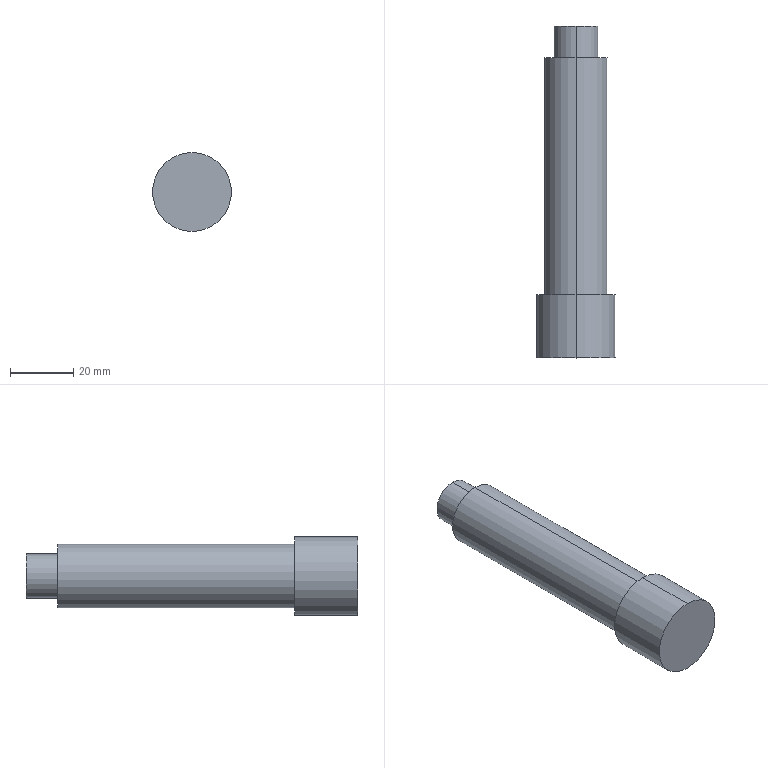Part | SolidWorks | features ICE 2, Extrusion 1 | 1 solid | 10 faces | box 25 x 105 x 25 mm | volume 34919 mm3 | cylinder 6 | plane 4 | commonest cylinder face diameters 14 x2 20 x2 25 x2
STEP:
#1=CARTESIAN_POINT('',(0.,105.,7.));
#2=VERTEX_POINT('',#1);
#3=CARTESIAN_POINT('',(0.,105.,-7.));
#4=VERTEX_POINT('',#3);
#5=CARTESIAN_POINT('',(0.,105.,0.));
#6=DIRECTION('',(0.,1.,0.));
#7=DIRECTION('',(0.,0.,1.));
#8=AXIS2_PLACEMENT_3D('',#5,#6,#7);
#9=CIRCLE('',#8,7.);
#10=EDGE_CURVE('',#2,#4,#9,.T.);
#11=ORIENTED_EDGE('',*,*,#10,.F.);
#12=CARTESIAN_POINT('',(0.,95.,7.));
#13=VERTEX_POINT('',#12);
#14=CARTESIAN_POINT('',(0.,105.,7.));
#15=DIRECTION('',(0.,-1.,0.));
#16=VECTOR('',#15,1000.);
#17=LINE('',#14,#16);
#18=EDGE_CURVE('',#2,#13,#17,.T.);
#19=ORIENTED_EDGE('',*,*,#18,.T.);
#20=CARTESIAN_POINT('',(0.,95.,-7.));
#21=VERTEX_POINT('',#20);
#22=CARTESIAN_POINT('',(0.,95.,0.));
#23=DIRECTION('',(0.,1.,0.));
#24=DIRECTION('',(0.,0.,1.));
#25=AXIS2_PLACEMENT_3D('',#22,#23,#24);
#26=CIRCLE('',#25,7.);
#27=EDGE_CURVE('',#13,#21,#26,.T.);
#28=ORIENTED_EDGE('',*,*,#27,.T.);
#29=CARTESIAN_POINT('',(0.,105.,-7.));
#30=DIRECTION('',(0.,-1.,0.));
#31=VECTOR('',#30,1000.);
#32=LINE('',#29,#31);
#33=EDGE_CURVE('',#4,#21,#32,.T.);
#34=ORIENTED_EDGE('',*,*,#33,.F.);
#35=EDGE_LOOP('',(#11,#19,#28,#34));
#36=FACE_OUTER_BOUND('',#35,.T.);
#37=CARTESIAN_POINT('',(0.,105.,0.));
#38=DIRECTION('',(0.,-1.,0.));
#39=DIRECTION('',(0.,0.,-1.));
#40=AXIS2_PLACEMENT_3D('',#37,#38,#39);
#41=CYLINDRICAL_SURFACE('',#40,7.);
#42=ADVANCED_FACE('',(#36),#41,.T.);
#43=CARTESIAN_POINT('',(0.,95.,10.));
#44=VERTEX_POINT('',#43);
#45=CARTESIAN_POINT('',(0.,95.,-10.));
#46=VERTEX_POINT('',#45);
#47=CARTESIAN_POINT('',(0.,95.,0.));
#48=DIRECTION('',(0.,1.,0.));
#49=DIRECTION('',(0.,0.,1.));
#50=AXIS2_PLACEMENT_3D('',#47,#48,#49);
#51=CIRCLE('',#50,10.);
#52=EDGE_CURVE('',#44,#46,#51,.T.);
#53=ORIENTED_EDGE('',*,*,#52,.F.);
#54=CARTESIAN_POINT('',(0.,20.,10.));
#55=VERTEX_POINT('',#54);
#56=CARTESIAN_POINT('',(0.,95.,10.));
#57=DIRECTION('',(0.,-1.,0.));
#58=VECTOR('',#57,1000.);
#59=LINE('',#56,#58);
#60=EDGE_CURVE('',#44,#55,#59,.T.);
#61=ORIENTED_EDGE('',*,*,#60,.T.);
#62=CARTESIAN_POINT('',(0.,20.,-10.));
#63=VERTEX_POINT('',#62);
#64=CARTESIAN_POINT('',(0.,20.,0.));
#65=DIRECTION('',(0.,1.,0.));
#66=DIRECTION('',(0.,0.,1.));
#67=AXIS2_PLACEMENT_3D('',#64,#65,#66);
#68=CIRCLE('',#67,10.);
#69=EDGE_CURVE('',#55,#63,#68,.T.);
#70=ORIENTED_EDGE('',*,*,#69,.T.);
#71=CARTESIAN_POINT('',(0.,95.,-10.));
#72=DIRECTION('',(0.,-1.,0.));
#73=VECTOR('',#72,1000.);
#74=LINE('',#71,#73);
#75=EDGE_CURVE('',#46,#63,#74,.T.);
#76=ORIENTED_EDGE('',*,*,#75,.F.);
#77=EDGE_LOOP('',(#53,#61,#70,#76));
#78=FACE_OUTER_BOUND('',#77,.T.);
#79=CARTESIAN_POINT('',(0.,95.,0.));
#80=DIRECTION('',(0.,-1.,0.));
#81=DIRECTION('',(0.,0.,-1.));
#82=AXIS2_PLACEMENT_3D('',#79,#80,#81);
#83=CYLINDRICAL_SURFACE('',#82,10.);
#84=ADVANCED_FACE('',(#78),#83,.T.);
#85=CARTESIAN_POINT('',(0.,20.,12.5));
#86=VERTEX_POINT('',#85);
#87=CARTESIAN_POINT('',(0.,20.,-12.5));
#88=VERTEX_POINT('',#87);
#89=CARTESIAN_POINT('',(0.,20.,0.));
#90=DIRECTION('',(0.,1.,0.));
#91=DIRECTION('',(0.,0.,1.));
#92=AXIS2_PLACEMENT_3D('',#89,#90,#91);
#93=CIRCLE('',#92,12.5);
#94=EDGE_CURVE('',#86,#88,#93,.T.);
#95=ORIENTED_EDGE('',*,*,#94,.F.);
#96=CARTESIAN_POINT('',(0.,0.,12.5));
#97=VERTEX_POINT('',#96);
#98=CARTESIAN_POINT('',(0.,20.,12.5));
#99=DIRECTION('',(0.,-1.,0.));
#100=VECTOR('',#99,1000.);
#101=LINE('',#98,#100);
#102=EDGE_CURVE('',#86,#97,#101,.T.);
#103=ORIENTED_EDGE('',*,*,#102,.T.);
#104=CARTESIAN_POINT('',(0.,0.,-12.5));
#105=VERTEX_POINT('',#104);
#106=CARTESIAN_POINT('',(0.,0.,0.));
#107=DIRECTION('',(0.,1.,0.));
#108=DIRECTION('',(0.,0.,1.));
#109=AXIS2_PLACEMENT_3D('',#106,#107,#108);
#110=CIRCLE('',#109,12.5);
#111=EDGE_CURVE('',#97,#105,#110,.T.);
#112=ORIENTED_EDGE('',*,*,#111,.T.);
#113=CARTESIAN_POINT('',(0.,20.,-12.5));
#114=DIRECTION('',(0.,-1.,0.));
#115=VECTOR('',#114,1000.);
#116=LINE('',#113,#115);
#117=EDGE_CURVE('',#88,#105,#116,.T.);
#118=ORIENTED_EDGE('',*,*,#117,.F.);
#119=EDGE_LOOP('',(#95,#103,#112,#118));
#120=FACE_OUTER_BOUND('',#119,.T.);
#121=CARTESIAN_POINT('',(0.,20.,0.));
#122=DIRECTION('',(0.,-1.,0.));
#123=DIRECTION('',(0.,0.,-1.));
#124=AXIS2_PLACEMENT_3D('',#121,#122,#123);
#125=CYLINDRICAL_SURFACE('',#124,12.5);
#126=ADVANCED_FACE('',(#120),#125,.T.);
#127=ORIENTED_EDGE('',*,*,#102,.F.);
#128=CARTESIAN_POINT('',(0.,20.,0.));
#129=DIRECTION('',(0.,1.,0.));
#130=DIRECTION('',(0.,0.,1.));
#131=AXIS2_PLACEMENT_3D('',#128,#129,#130);
#132=CIRCLE('',#131,12.5);
#133=EDGE_CURVE('',#88,#86,#132,.T.);
#134=ORIENTED_EDGE('',*,*,#133,.F.);
#135=ORIENTED_EDGE('',*,*,#117,.T.);
#136=CARTESIAN_POINT('',(0.,0.,0.));
#137=DIRECTION('',(0.,1.,0.));
#138=DIRECTION('',(0.,0.,1.));
#139=AXIS2_PLACEMENT_3D('',#136,#137,#138);
#140=CIRCLE('',#139,12.5);
#141=EDGE_CURVE('',#105,#97,#140,.T.);
#142=ORIENTED_EDGE('',*,*,#141,.T.);
#143=EDGE_LOOP('',(#127,#134,#135,#142));
#144=FACE_OUTER_BOUND('',#143,.T.);
#145=CARTESIAN_POINT('',(0.,20.,0.));
#146=DIRECTION('',(0.,-1.,0.));
#147=DIRECTION('',(0.,0.,-1.));
#148=AXIS2_PLACEMENT_3D('',#145,#146,#147);
#149=CYLINDRICAL_SURFACE('',#148,12.5);
#150=ADVANCED_FACE('',(#144),#149,.T.);
#151=CARTESIAN_POINT('',(0.,20.,0.));
#152=DIRECTION('',(0.,1.,0.));
#153=DIRECTION('',(0.,0.,1.));
#154=AXIS2_PLACEMENT_3D('',#151,#152,#153);
#155=CIRCLE('',#154,10.);
#156=EDGE_CURVE('',#63,#55,#155,.T.);
#157=ORIENTED_EDGE('',*,*,#156,.F.);
#158=ORIENTED_EDGE('',*,*,#69,.F.);
#159=EDGE_LOOP('',(#157,#158));
#160=FACE_BOUND('',#159,.T.);
#161=ORIENTED_EDGE('',*,*,#133,.T.);
#162=ORIENTED_EDGE('',*,*,#94,.T.);
#163=EDGE_LOOP('',(#161,#162));
#164=FACE_OUTER_BOUND('',#163,.T.);
#165=CARTESIAN_POINT('',(0.,20.,0.));
#166=DIRECTION('',(0.,1.,0.));
#167=DIRECTION('',(0.,0.,1.));
#168=AXIS2_PLACEMENT_3D('',#165,#166,#167);
#169=PLANE('',#168);
#170=ADVANCED_FACE('',(#160,#164),#169,.T.);
#171=ORIENTED_EDGE('',*,*,#141,.F.);
#172=ORIENTED_EDGE('',*,*,#111,.F.);
#173=EDGE_LOOP('',(#171,#172));
#174=FACE_OUTER_BOUND('',#173,.T.);
#175=CARTESIAN_POINT('',(0.,0.,0.));
#176=DIRECTION('',(0.,1.,0.));
#177=DIRECTION('',(0.,0.,1.));
#178=AXIS2_PLACEMENT_3D('',#175,#176,#177);
#179=PLANE('',#178);
#180=ADVANCED_FACE('',(#174),#179,.F.);
#181=ORIENTED_EDGE('',*,*,#60,.F.);
#182=CARTESIAN_POINT('',(0.,95.,0.));
#183=DIRECTION('',(0.,1.,0.));
#184=DIRECTION('',(0.,0.,1.));
#185=AXIS2_PLACEMENT_3D('',#182,#183,#184);
#186=CIRCLE('',#185,10.);
#187=EDGE_CURVE('',#46,#44,#186,.T.);
#188=ORIENTED_EDGE('',*,*,#187,.F.);
#189=ORIENTED_EDGE('',*,*,#75,.T.);
#190=ORIENTED_EDGE('',*,*,#156,.T.);
#191=EDGE_LOOP('',(#181,#188,#189,#190));
#192=FACE_OUTER_BOUND('',#191,.T.);
#193=CARTESIAN_POINT('',(0.,95.,0.));
#194=DIRECTION('',(0.,-1.,0.));
#195=DIRECTION('',(0.,0.,-1.));
#196=AXIS2_PLACEMENT_3D('',#193,#194,#195);
#197=CYLINDRICAL_SURFACE('',#196,10.);
#198=ADVANCED_FACE('',(#192),#197,.T.);
#199=CARTESIAN_POINT('',(0.,95.,0.));
#200=DIRECTION('',(0.,1.,0.));
#201=DIRECTION('',(0.,0.,1.));
#202=AXIS2_PLACEMENT_3D('',#199,#200,#201);
#203=CIRCLE('',#202,7.);
#204=EDGE_CURVE('',#21,#13,#203,.T.);
#205=ORIENTED_EDGE('',*,*,#204,.F.);
#206=ORIENTED_EDGE('',*,*,#27,.F.);
#207=EDGE_LOOP('',(#205,#206));
#208=FACE_BOUND('',#207,.T.);
#209=ORIENTED_EDGE('',*,*,#187,.T.);
#210=ORIENTED_EDGE('',*,*,#52,.T.);
#211=EDGE_LOOP('',(#209,#210));
#212=FACE_OUTER_BOUND('',#211,.T.);
#213=CARTESIAN_POINT('',(0.,95.,0.));
#214=DIRECTION('',(0.,1.,0.));
#215=DIRECTION('',(0.,0.,1.));
#216=AXIS2_PLACEMENT_3D('',#213,#214,#215);
#217=PLANE('',#216);
#218=ADVANCED_FACE('',(#208,#212),#217,.T.);
#219=ORIENTED_EDGE('',*,*,#18,.F.);
#220=CARTESIAN_POINT('',(0.,105.,0.));
#221=DIRECTION('',(0.,1.,0.));
#222=DIRECTION('',(0.,0.,1.));
#223=AXIS2_PLACEMENT_3D('',#220,#221,#222);
#224=CIRCLE('',#223,7.);
#225=EDGE_CURVE('',#4,#2,#224,.T.);
#226=ORIENTED_EDGE('',*,*,#225,.F.);
#227=ORIENTED_EDGE('',*,*,#33,.T.);
#228=ORIENTED_EDGE('',*,*,#204,.T.);
#229=EDGE_LOOP('',(#219,#226,#227,#228));
#230=FACE_OUTER_BOUND('',#229,.T.);
#231=CARTESIAN_POINT('',(0.,105.,0.));
#232=DIRECTION('',(0.,-1.,0.));
#233=DIRECTION('',(0.,0.,-1.));
#234=AXIS2_PLACEMENT_3D('',#231,#232,#233);
#235=CYLINDRICAL_SURFACE('',#234,7.);
#236=ADVANCED_FACE('',(#230),#235,.T.);
#237=ORIENTED_EDGE('',*,*,#225,.T.);
#238=ORIENTED_EDGE('',*,*,#10,.T.);
#239=EDGE_LOOP('',(#237,#238));
#240=FACE_OUTER_BOUND('',#239,.T.);
#241=CARTESIAN_POINT('',(0.,105.,0.));
#242=DIRECTION('',(0.,1.,0.));
#243=DIRECTION('',(0.,0.,1.));
#244=AXIS2_PLACEMENT_3D('',#241,#242,#243);
#245=PLANE('',#244);
#246=ADVANCED_FACE('',(#240),#245,.T.);
#247=CLOSED_SHELL('',(#42,#84,#126,#150,#170,#180,#198,#218,#236,#246));
#248=MANIFOLD_SOLID_BREP('',#247);
#249=CARTESIAN_POINT('',(0.,0.,0.));
#250=DIRECTION('',(0.,0.,1.));
#251=DIRECTION('',(1.,0.,0.));
#252=AXIS2_PLACEMENT_3D('',#249,#250,#251);
#253=(LENGTH_UNIT()NAMED_UNIT(*)SI_UNIT(.MILLI.,.METRE.));
#254=UNCERTAINTY_MEASURE_WITH_UNIT(LENGTH_MEASURE(0.00001),#253,'','');
#255=(NAMED_UNIT(*)PLANE_ANGLE_UNIT()SI_UNIT($,.RADIAN.));
#256=(NAMED_UNIT(*)SI_UNIT($,.STERADIAN.)SOLID_ANGLE_UNIT());
#257=(GEOMETRIC_REPRESENTATION_CONTEXT(3)GLOBAL_UNCERTAINTY_ASSIGNED_CONTEXT((#254))GLOBAL_UNIT_ASSIGNED_CONTEXT((#253,#255,#256))REPRESENTATION_CONTEXT('',''));
#258=ADVANCED_BREP_SHAPE_REPRESENTATION('',(#248,#252),#257);